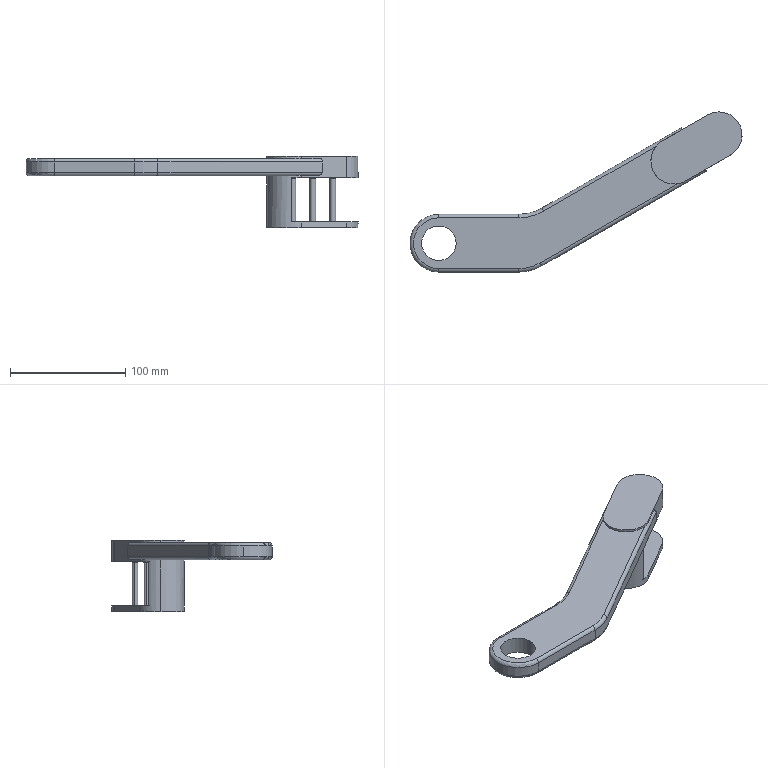Part | SolidWorks | features ICE 4, Extrusion 1, Fillet 1, LPattern 1 | 1 solid | 54 faces | box 287.553 x 138.722 x 62 mm | volume 231304 mm3 | cylinder 28 | plane 20 | torus 6 | commonest cylinder face diameters 6 x10 5 x6 40 x6 30 x2 50 x2 80 x2